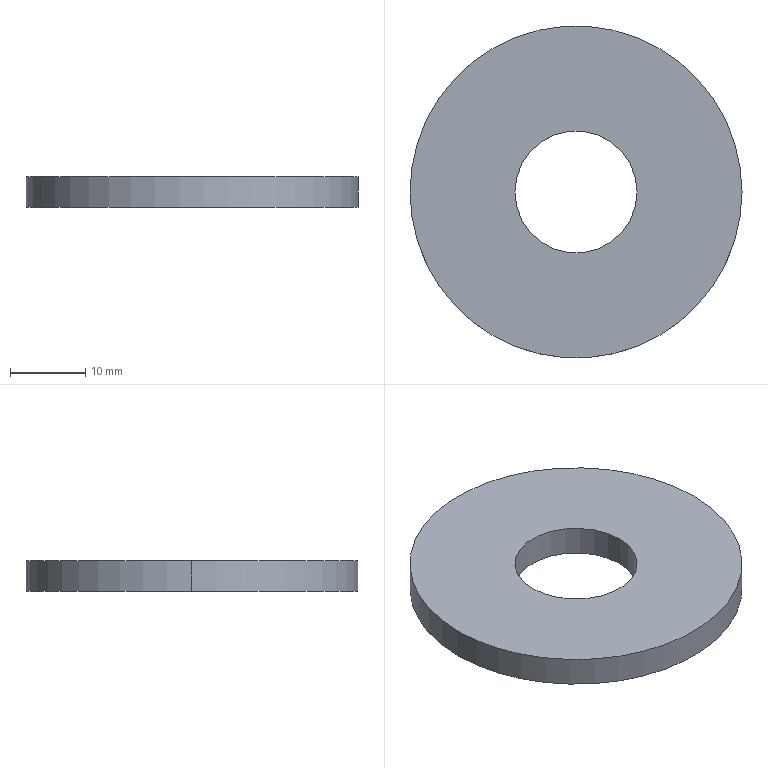Part | SolidWorks | features Extrusion 1 | 1 solid | 6 faces | box 44 x 44 x 4 mm | volume 5258 mm3 | cylinder 4 | plane 2 | commonest cylinder face diameters 16.2 x2 44 x2
STEP:
#1=CARTESIAN_POINT('',(-8.1,0.,-2.));
#2=VERTEX_POINT('',#1);
#3=CARTESIAN_POINT('',(8.1,0.,-2.));
#4=VERTEX_POINT('',#3);
#5=CARTESIAN_POINT('',(0.,0.,-2.));
#6=DIRECTION('',(0.,0.,1.));
#7=DIRECTION('',(1.,0.,0.));
#8=AXIS2_PLACEMENT_3D('',#5,#6,#7);
#9=CIRCLE('',#8,8.1);
#10=EDGE_CURVE('',#2,#4,#9,.T.);
#11=ORIENTED_EDGE('',*,*,#10,.F.);
#12=CARTESIAN_POINT('',(-8.1,0.,2.));
#13=VERTEX_POINT('',#12);
#14=CARTESIAN_POINT('',(-8.1,0.,-2.));
#15=DIRECTION('',(0.,0.,1.));
#16=VECTOR('',#15,1000.);
#17=LINE('',#14,#16);
#18=EDGE_CURVE('',#2,#13,#17,.T.);
#19=ORIENTED_EDGE('',*,*,#18,.T.);
#20=CARTESIAN_POINT('',(8.1,0.,2.));
#21=VERTEX_POINT('',#20);
#22=CARTESIAN_POINT('',(0.,0.,2.));
#23=DIRECTION('',(0.,0.,1.));
#24=DIRECTION('',(1.,0.,0.));
#25=AXIS2_PLACEMENT_3D('',#22,#23,#24);
#26=CIRCLE('',#25,8.1);
#27=EDGE_CURVE('',#13,#21,#26,.T.);
#28=ORIENTED_EDGE('',*,*,#27,.T.);
#29=CARTESIAN_POINT('',(8.1,0.,-2.));
#30=DIRECTION('',(0.,0.,1.));
#31=VECTOR('',#30,1000.);
#32=LINE('',#29,#31);
#33=EDGE_CURVE('',#4,#21,#32,.T.);
#34=ORIENTED_EDGE('',*,*,#33,.F.);
#35=EDGE_LOOP('',(#11,#19,#28,#34));
#36=FACE_OUTER_BOUND('',#35,.T.);
#37=CARTESIAN_POINT('',(0.,0.,-2.));
#38=DIRECTION('',(0.,0.,1.));
#39=DIRECTION('',(1.,0.,0.));
#40=AXIS2_PLACEMENT_3D('',#37,#38,#39);
#41=CYLINDRICAL_SURFACE('',#40,8.1);
#42=ADVANCED_FACE('',(#36),#41,.F.);
#43=CARTESIAN_POINT('',(22.,0.,-2.));
#44=VERTEX_POINT('',#43);
#45=CARTESIAN_POINT('',(-22.,0.,-2.));
#46=VERTEX_POINT('',#45);
#47=CARTESIAN_POINT('',(0.,0.,-2.));
#48=DIRECTION('',(0.,0.,1.));
#49=DIRECTION('',(1.,0.,0.));
#50=AXIS2_PLACEMENT_3D('',#47,#48,#49);
#51=CIRCLE('',#50,22.);
#52=EDGE_CURVE('',#44,#46,#51,.T.);
#53=ORIENTED_EDGE('',*,*,#52,.T.);
#54=CARTESIAN_POINT('',(-22.,0.,2.));
#55=VERTEX_POINT('',#54);
#56=CARTESIAN_POINT('',(-22.,0.,-2.));
#57=DIRECTION('',(0.,0.,1.));
#58=VECTOR('',#57,1000.);
#59=LINE('',#56,#58);
#60=EDGE_CURVE('',#46,#55,#59,.T.);
#61=ORIENTED_EDGE('',*,*,#60,.T.);
#62=CARTESIAN_POINT('',(22.,0.,2.));
#63=VERTEX_POINT('',#62);
#64=CARTESIAN_POINT('',(0.,0.,2.));
#65=DIRECTION('',(0.,0.,1.));
#66=DIRECTION('',(1.,0.,0.));
#67=AXIS2_PLACEMENT_3D('',#64,#65,#66);
#68=CIRCLE('',#67,22.);
#69=EDGE_CURVE('',#63,#55,#68,.T.);
#70=ORIENTED_EDGE('',*,*,#69,.F.);
#71=CARTESIAN_POINT('',(22.,0.,-2.));
#72=DIRECTION('',(0.,0.,1.));
#73=VECTOR('',#72,1000.);
#74=LINE('',#71,#73);
#75=EDGE_CURVE('',#44,#63,#74,.T.);
#76=ORIENTED_EDGE('',*,*,#75,.F.);
#77=EDGE_LOOP('',(#53,#61,#70,#76));
#78=FACE_OUTER_BOUND('',#77,.T.);
#79=CARTESIAN_POINT('',(0.,0.,-2.));
#80=DIRECTION('',(0.,0.,1.));
#81=DIRECTION('',(1.,0.,0.));
#82=AXIS2_PLACEMENT_3D('',#79,#80,#81);
#83=CYLINDRICAL_SURFACE('',#82,22.);
#84=ADVANCED_FACE('',(#78),#83,.T.);
#85=ORIENTED_EDGE('',*,*,#60,.F.);
#86=CARTESIAN_POINT('',(0.,0.,-2.));
#87=DIRECTION('',(0.,0.,1.));
#88=DIRECTION('',(1.,0.,0.));
#89=AXIS2_PLACEMENT_3D('',#86,#87,#88);
#90=CIRCLE('',#89,22.);
#91=EDGE_CURVE('',#46,#44,#90,.T.);
#92=ORIENTED_EDGE('',*,*,#91,.T.);
#93=ORIENTED_EDGE('',*,*,#75,.T.);
#94=CARTESIAN_POINT('',(0.,0.,2.));
#95=DIRECTION('',(0.,0.,1.));
#96=DIRECTION('',(1.,0.,0.));
#97=AXIS2_PLACEMENT_3D('',#94,#95,#96);
#98=CIRCLE('',#97,22.);
#99=EDGE_CURVE('',#55,#63,#98,.T.);
#100=ORIENTED_EDGE('',*,*,#99,.F.);
#101=EDGE_LOOP('',(#85,#92,#93,#100));
#102=FACE_OUTER_BOUND('',#101,.T.);
#103=CARTESIAN_POINT('',(0.,0.,-2.));
#104=DIRECTION('',(0.,0.,1.));
#105=DIRECTION('',(1.,0.,0.));
#106=AXIS2_PLACEMENT_3D('',#103,#104,#105);
#107=CYLINDRICAL_SURFACE('',#106,22.);
#108=ADVANCED_FACE('',(#102),#107,.T.);
#109=CARTESIAN_POINT('',(0.,0.,-2.));
#110=DIRECTION('',(0.,0.,1.));
#111=DIRECTION('',(1.,0.,0.));
#112=AXIS2_PLACEMENT_3D('',#109,#110,#111);
#113=CIRCLE('',#112,8.1);
#114=EDGE_CURVE('',#4,#2,#113,.T.);
#115=ORIENTED_EDGE('',*,*,#114,.T.);
#116=ORIENTED_EDGE('',*,*,#10,.T.);
#117=EDGE_LOOP('',(#115,#116));
#118=FACE_BOUND('',#117,.T.);
#119=ORIENTED_EDGE('',*,*,#52,.F.);
#120=ORIENTED_EDGE('',*,*,#91,.F.);
#121=EDGE_LOOP('',(#119,#120));
#122=FACE_OUTER_BOUND('',#121,.T.);
#123=CARTESIAN_POINT('',(0.,0.,-2.));
#124=DIRECTION('',(0.,0.,1.));
#125=DIRECTION('',(1.,0.,0.));
#126=AXIS2_PLACEMENT_3D('',#123,#124,#125);
#127=PLANE('',#126);
#128=ADVANCED_FACE('',(#118,#122),#127,.F.);
#129=CARTESIAN_POINT('',(0.,0.,2.));
#130=DIRECTION('',(0.,0.,1.));
#131=DIRECTION('',(1.,0.,0.));
#132=AXIS2_PLACEMENT_3D('',#129,#130,#131);
#133=CIRCLE('',#132,8.1);
#134=EDGE_CURVE('',#21,#13,#133,.T.);
#135=ORIENTED_EDGE('',*,*,#134,.F.);
#136=ORIENTED_EDGE('',*,*,#27,.F.);
#137=EDGE_LOOP('',(#135,#136));
#138=FACE_BOUND('',#137,.T.);
#139=ORIENTED_EDGE('',*,*,#69,.T.);
#140=ORIENTED_EDGE('',*,*,#99,.T.);
#141=EDGE_LOOP('',(#139,#140));
#142=FACE_OUTER_BOUND('',#141,.T.);
#143=CARTESIAN_POINT('',(0.,0.,2.));
#144=DIRECTION('',(0.,0.,1.));
#145=DIRECTION('',(1.,0.,0.));
#146=AXIS2_PLACEMENT_3D('',#143,#144,#145);
#147=PLANE('',#146);
#148=ADVANCED_FACE('',(#138,#142),#147,.T.);
#149=ORIENTED_EDGE('',*,*,#18,.F.);
#150=ORIENTED_EDGE('',*,*,#114,.F.);
#151=ORIENTED_EDGE('',*,*,#33,.T.);
#152=ORIENTED_EDGE('',*,*,#134,.T.);
#153=EDGE_LOOP('',(#149,#150,#151,#152));
#154=FACE_OUTER_BOUND('',#153,.T.);
#155=CARTESIAN_POINT('',(0.,0.,-2.));
#156=DIRECTION('',(0.,0.,1.));
#157=DIRECTION('',(1.,0.,0.));
#158=AXIS2_PLACEMENT_3D('',#155,#156,#157);
#159=CYLINDRICAL_SURFACE('',#158,8.1);
#160=ADVANCED_FACE('',(#154),#159,.F.);
#161=CLOSED_SHELL('',(#42,#84,#108,#128,#148,#160));
#162=MANIFOLD_SOLID_BREP('',#161);
#163=CARTESIAN_POINT('',(0.,0.,0.));
#164=DIRECTION('',(0.,0.,1.));
#165=DIRECTION('',(1.,0.,0.));
#166=AXIS2_PLACEMENT_3D('',#163,#164,#165);
#167=(LENGTH_UNIT()NAMED_UNIT(*)SI_UNIT(.MILLI.,.METRE.));
#168=UNCERTAINTY_MEASURE_WITH_UNIT(LENGTH_MEASURE(0.00001),#167,'','');
#169=(NAMED_UNIT(*)PLANE_ANGLE_UNIT()SI_UNIT($,.RADIAN.));
#170=(NAMED_UNIT(*)SI_UNIT($,.STERADIAN.)SOLID_ANGLE_UNIT());
#171=(GEOMETRIC_REPRESENTATION_CONTEXT(3)GLOBAL_UNCERTAINTY_ASSIGNED_CONTEXT((#168))GLOBAL_UNIT_ASSIGNED_CONTEXT((#167,#169,#170))REPRESENTATION_CONTEXT('',''));
#172=ADVANCED_BREP_SHAPE_REPRESENTATION('',(#162,#166),#171);